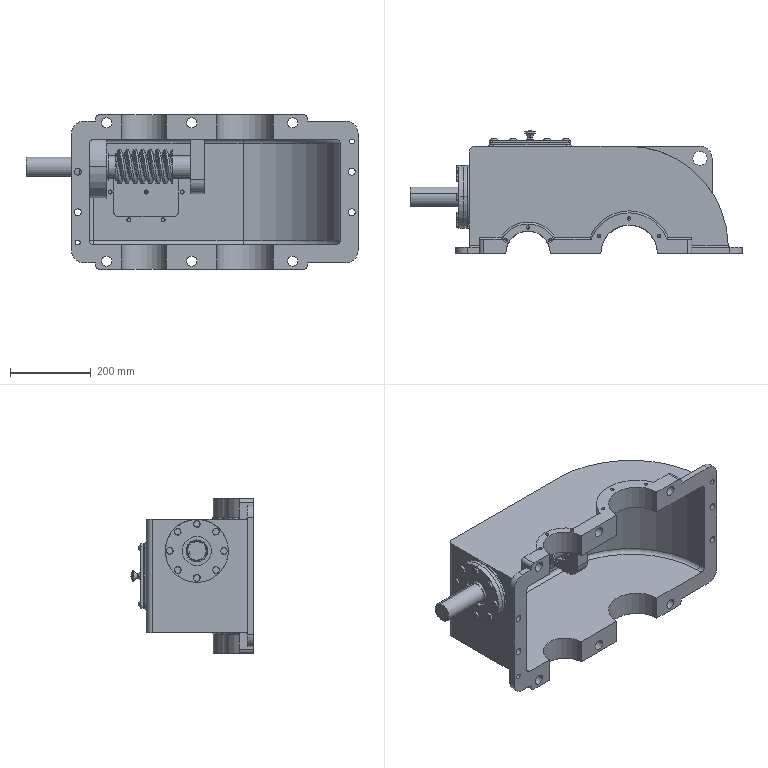Part | SolidWorks | features CompositeCurve 13 | 38 solids | 2960 faces | box 820.75 x 304 x 382 mm | volume 10937552 mm3 | cylinder 1282 | cone 730 | plane 595 | torus 214 | sphere 111 | spline 28 | commonest cylinder face diameters 10 x731 0.5 x153 25 x112 8.5 x66 20 x20 84 x18